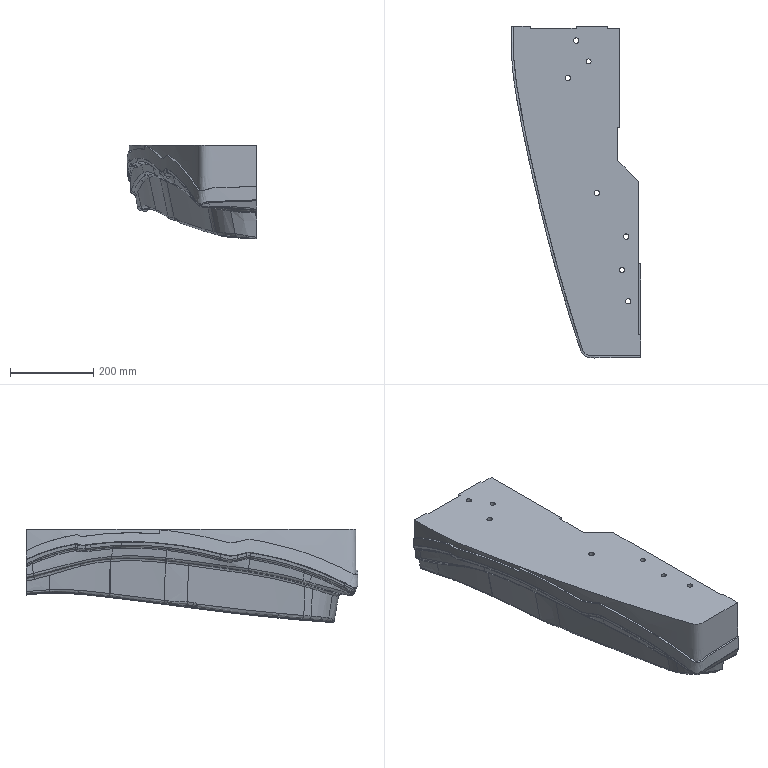Part | NX | features solid 2 | 1 solid | 268 faces | box 310.261 x 795.79 x 223.576 mm | volume 23666276 mm3 | spline 224 | plane 29 | cylinder 15 | commonest cylinder face diameters 13 x7 20 x5 12 x2 30 x1